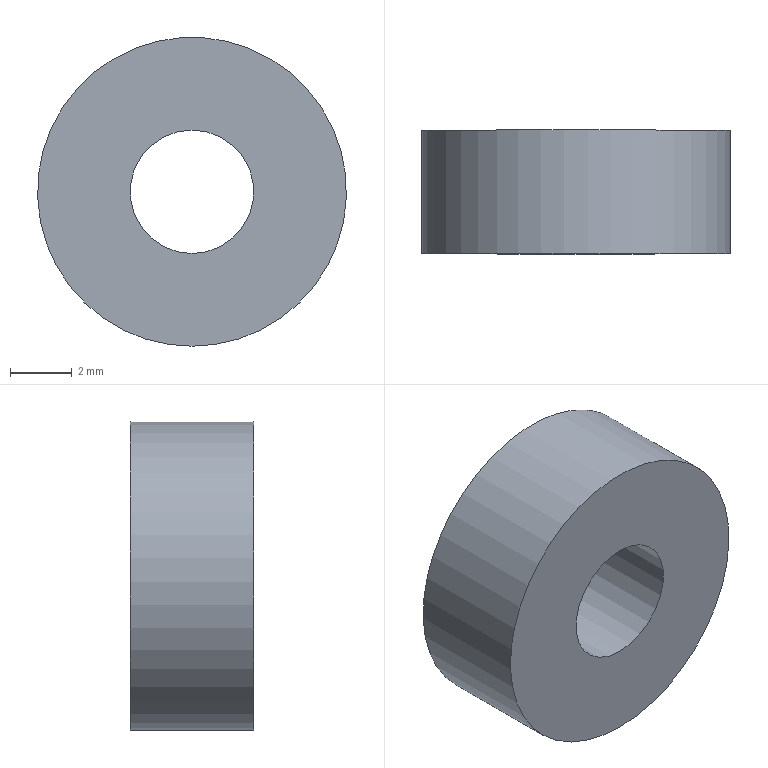Part | STEP file | Dodanie-wyci_gni_cie1 | 1 solid | 4 faces | box 10 x 4 x 10 mm | volume 263.894 mm3 | cylinder 2 | plane 2 | commonest cylinder face diameters 4 x1 10 x1
STEP:
#1=CARTESIAN_POINT('',(0.,0.,0.));
#2=DIRECTION('',(0.,0.,1.));
#3=DIRECTION('',(1.,0.,0.));
#4=AXIS2_PLACEMENT_3D('',#1,#2,#3);
#5=CARTESIAN_POINT('',(-99.682,73.388,-112.798));
#6=VERTEX_POINT('',#5);
#7=CARTESIAN_POINT('',(-99.682,69.388,-112.798));
#8=VERTEX_POINT('',#7);
#9=CARTESIAN_POINT('',(-99.682,73.388,-112.798));
#10=DIRECTION('',(0.,-1.,0.));
#11=VECTOR('',#10,1.);
#12=LINE('',#9,#11);
#13=CARTESIAN_POINT('',(-99.682,69.388,-107.798));
#14=DIRECTION('',(0.,1.,0.));
#15=DIRECTION('',(0.,0.,-1.));
#16=AXIS2_PLACEMENT_3D('',#13,#14,#15);
#17=CYLINDRICAL_SURFACE('',#16,5.);
#18=CARTESIAN_POINT('',(0.,4.));
#19=DIRECTION('',(0.,-1.));
#20=VECTOR('',#19,1.);
#21=LINE('',#18,#20);
#22=(GEOMETRIC_REPRESENTATION_CONTEXT(2)PARAMETRIC_REPRESENTATION_CONTEXT()REPRESENTATION_CONTEXT('',''));
#23=DEFINITIONAL_REPRESENTATION('',(#21),#22);
#24=PCURVE('',#17,#23);
#25=CARTESIAN_POINT('',(6.283,4.));
#26=DIRECTION('',(0.,-1.));
#27=VECTOR('',#26,1.);
#28=LINE('',#25,#27);
#29=(GEOMETRIC_REPRESENTATION_CONTEXT(2)PARAMETRIC_REPRESENTATION_CONTEXT()REPRESENTATION_CONTEXT('',''));
#30=DEFINITIONAL_REPRESENTATION('',(#28),#29);
#31=PCURVE('',#17,#30);
#32=SEAM_CURVE('',#12,(#24,#31),.PCURVE_S1.);
#33=EDGE_CURVE('',#6,#8,#32,.T.);
#34=ORIENTED_EDGE('',*,*,#33,.T.);
#35=CARTESIAN_POINT('',(-99.682,69.388,-107.798));
#36=DIRECTION('',(0.,1.,0.));
#37=DIRECTION('',(0.,0.,-1.));
#38=AXIS2_PLACEMENT_3D('',#35,#36,#37);
#39=CIRCLE('',#38,5.);
#40=CARTESIAN_POINT('',(0.,0.));
#41=DIRECTION('',(1.,0.));
#42=VECTOR('',#41,1.);
#43=LINE('',#40,#42);
#44=(GEOMETRIC_REPRESENTATION_CONTEXT(2)PARAMETRIC_REPRESENTATION_CONTEXT()REPRESENTATION_CONTEXT('',''));
#45=DEFINITIONAL_REPRESENTATION('',(#43),#44);
#46=PCURVE('',#17,#45);
#47=CARTESIAN_POINT('',(-99.682,69.388,-107.798));
#48=DIRECTION('',(0.,-1.,0.));
#49=DIRECTION('',(0.,0.,1.));
#50=AXIS2_PLACEMENT_3D('',#47,#48,#49);
#51=PLANE('',#50);
#52=CARTESIAN_POINT('',(-5.,0.));
#53=CARTESIAN_POINT('',(-5.,8.66));
#54=CARTESIAN_POINT('',(2.5,4.33));
#55=CARTESIAN_POINT('',(10.,0.));
#56=CARTESIAN_POINT('',(2.5,-4.33));
#57=CARTESIAN_POINT('',(-5.,-8.66));
#58=CARTESIAN_POINT('',(-5.,0.));
#59=(BOUNDED_CURVE()B_SPLINE_CURVE(2,(#52,#53,#54,#55,#56,#57,#58),.UNSPECIFIED.,.T.,.F.)B_SPLINE_CURVE_WITH_KNOTS((1,2,2,2,2,1),(-2.094,0.,2.094,4.189,6.283,8.378),.UNSPECIFIED.)CURVE()GEOMETRIC_REPRESENTATION_ITEM()RATIONAL_B_SPLINE_CURVE((1.,0.5,1.,0.5,1.,0.5,1.))REPRESENTATION_ITEM(''));
#60=(GEOMETRIC_REPRESENTATION_CONTEXT(2)PARAMETRIC_REPRESENTATION_CONTEXT()REPRESENTATION_CONTEXT('',''));
#61=DEFINITIONAL_REPRESENTATION('',(#59),#60);
#62=PCURVE('',#51,#61);
#63=SURFACE_CURVE('',#39,(#46,#62),.PCURVE_S1.);
#64=EDGE_CURVE('',#8,#8,#63,.T.);
#65=ORIENTED_EDGE('',*,*,#64,.T.);
#66=ORIENTED_EDGE('',*,*,#33,.F.);
#67=CARTESIAN_POINT('',(-99.682,73.388,-107.798));
#68=DIRECTION('',(0.,-1.,0.));
#69=DIRECTION('',(0.,0.,-1.));
#70=AXIS2_PLACEMENT_3D('',#67,#68,#69);
#71=CIRCLE('',#70,5.);
#72=CARTESIAN_POINT('',(6.283,4.));
#73=DIRECTION('',(-1.,0.));
#74=VECTOR('',#73,1.);
#75=LINE('',#72,#74);
#76=(GEOMETRIC_REPRESENTATION_CONTEXT(2)PARAMETRIC_REPRESENTATION_CONTEXT()REPRESENTATION_CONTEXT('',''));
#77=DEFINITIONAL_REPRESENTATION('',(#75),#76);
#78=PCURVE('',#17,#77);
#79=CARTESIAN_POINT('',(-99.682,73.388,-107.798));
#80=DIRECTION('',(0.,-1.,0.));
#81=DIRECTION('',(0.,0.,1.));
#82=AXIS2_PLACEMENT_3D('',#79,#80,#81);
#83=PLANE('',#82);
#84=CARTESIAN_POINT('',(0.,0.));
#85=DIRECTION('',(-1.,0.));
#86=AXIS2_PLACEMENT_2D('',#84,#85);
#87=CIRCLE('',#86,5.);
#88=(GEOMETRIC_REPRESENTATION_CONTEXT(2)PARAMETRIC_REPRESENTATION_CONTEXT()REPRESENTATION_CONTEXT('',''));
#89=DEFINITIONAL_REPRESENTATION('',(#87),#88);
#90=PCURVE('',#83,#89);
#91=SURFACE_CURVE('',#71,(#78,#90),.PCURVE_S1.);
#92=EDGE_CURVE('',#6,#6,#91,.T.);
#93=ORIENTED_EDGE('',*,*,#92,.T.);
#94=EDGE_LOOP('',(#34,#65,#66,#93));
#95=FACE_BOUND('',#94,.T.);
#96=ADVANCED_FACE('',(#95),#17,.T.);
#97=CARTESIAN_POINT('',(-99.682,69.388,-109.798));
#98=VERTEX_POINT('',#97);
#99=CARTESIAN_POINT('',(-99.682,69.388,-107.798));
#100=DIRECTION('',(0.,1.,0.));
#101=DIRECTION('',(0.,0.,-1.));
#102=AXIS2_PLACEMENT_3D('',#99,#100,#101);
#103=CIRCLE('',#102,2.);
#104=CARTESIAN_POINT('',(-99.682,69.388,-107.798));
#105=DIRECTION('',(0.,1.,0.));
#106=DIRECTION('',(0.,0.,-1.));
#107=AXIS2_PLACEMENT_3D('',#104,#105,#106);
#108=CYLINDRICAL_SURFACE('',#107,2.);
#109=CARTESIAN_POINT('',(0.,0.));
#110=DIRECTION('',(1.,0.));
#111=VECTOR('',#110,1.);
#112=LINE('',#109,#111);
#113=(GEOMETRIC_REPRESENTATION_CONTEXT(2)PARAMETRIC_REPRESENTATION_CONTEXT()REPRESENTATION_CONTEXT('',''));
#114=DEFINITIONAL_REPRESENTATION('',(#112),#113);
#115=PCURVE('',#108,#114);
#116=CARTESIAN_POINT('',(-2.,0.));
#117=CARTESIAN_POINT('',(-2.,3.464));
#118=CARTESIAN_POINT('',(1.,1.732));
#119=CARTESIAN_POINT('',(4.,0.));
#120=CARTESIAN_POINT('',(1.,-1.732));
#121=CARTESIAN_POINT('',(-2.,-3.464));
#122=CARTESIAN_POINT('',(-2.,0.));
#123=(BOUNDED_CURVE()B_SPLINE_CURVE(2,(#116,#117,#118,#119,#120,#121,#122),.UNSPECIFIED.,.T.,.F.)B_SPLINE_CURVE_WITH_KNOTS((1,2,2,2,2,1),(-2.094,0.,2.094,4.189,6.283,8.378),.UNSPECIFIED.)CURVE()GEOMETRIC_REPRESENTATION_ITEM()RATIONAL_B_SPLINE_CURVE((1.,0.5,1.,0.5,1.,0.5,1.))REPRESENTATION_ITEM(''));
#124=(GEOMETRIC_REPRESENTATION_CONTEXT(2)PARAMETRIC_REPRESENTATION_CONTEXT()REPRESENTATION_CONTEXT('',''));
#125=DEFINITIONAL_REPRESENTATION('',(#123),#124);
#126=PCURVE('',#51,#125);
#127=SURFACE_CURVE('',#103,(#115,#126),.PCURVE_S1.);
#128=EDGE_CURVE('',#98,#98,#127,.T.);
#129=ORIENTED_EDGE('',*,*,#128,.T.);
#130=CARTESIAN_POINT('',(-99.682,73.388,-109.798));
#131=VERTEX_POINT('',#130);
#132=CARTESIAN_POINT('',(-99.682,73.388,-109.798));
#133=DIRECTION('',(0.,-1.,0.));
#134=VECTOR('',#133,1.);
#135=LINE('',#132,#134);
#136=CARTESIAN_POINT('',(6.283,4.));
#137=DIRECTION('',(0.,-1.));
#138=VECTOR('',#137,1.);
#139=LINE('',#136,#138);
#140=(GEOMETRIC_REPRESENTATION_CONTEXT(2)PARAMETRIC_REPRESENTATION_CONTEXT()REPRESENTATION_CONTEXT('',''));
#141=DEFINITIONAL_REPRESENTATION('',(#139),#140);
#142=PCURVE('',#108,#141);
#143=CARTESIAN_POINT('',(0.,4.));
#144=DIRECTION('',(0.,-1.));
#145=VECTOR('',#144,1.);
#146=LINE('',#143,#145);
#147=(GEOMETRIC_REPRESENTATION_CONTEXT(2)PARAMETRIC_REPRESENTATION_CONTEXT()REPRESENTATION_CONTEXT('',''));
#148=DEFINITIONAL_REPRESENTATION('',(#146),#147);
#149=PCURVE('',#108,#148);
#150=SEAM_CURVE('',#135,(#142,#149),.PCURVE_S1.);
#151=EDGE_CURVE('',#131,#98,#150,.T.);
#152=ORIENTED_EDGE('',*,*,#151,.F.);
#153=CARTESIAN_POINT('',(-99.682,73.388,-107.798));
#154=DIRECTION('',(0.,1.,0.));
#155=DIRECTION('',(0.,0.,-1.));
#156=AXIS2_PLACEMENT_3D('',#153,#154,#155);
#157=CIRCLE('',#156,2.);
#158=CARTESIAN_POINT('',(0.,4.));
#159=DIRECTION('',(1.,0.));
#160=VECTOR('',#159,1.);
#161=LINE('',#158,#160);
#162=(GEOMETRIC_REPRESENTATION_CONTEXT(2)PARAMETRIC_REPRESENTATION_CONTEXT()REPRESENTATION_CONTEXT('',''));
#163=DEFINITIONAL_REPRESENTATION('',(#161),#162);
#164=PCURVE('',#108,#163);
#165=CARTESIAN_POINT('',(-2.,0.));
#166=CARTESIAN_POINT('',(-2.,3.464));
#167=CARTESIAN_POINT('',(1.,1.732));
#168=CARTESIAN_POINT('',(4.,0.));
#169=CARTESIAN_POINT('',(1.,-1.732));
#170=CARTESIAN_POINT('',(-2.,-3.464));
#171=CARTESIAN_POINT('',(-2.,0.));
#172=(BOUNDED_CURVE()B_SPLINE_CURVE(2,(#165,#166,#167,#168,#169,#170,#171),.UNSPECIFIED.,.T.,.F.)B_SPLINE_CURVE_WITH_KNOTS((1,2,2,2,2,1),(-2.094,0.,2.094,4.189,6.283,8.378),.UNSPECIFIED.)CURVE()GEOMETRIC_REPRESENTATION_ITEM()RATIONAL_B_SPLINE_CURVE((1.,0.5,1.,0.5,1.,0.5,1.))REPRESENTATION_ITEM(''));
#173=(GEOMETRIC_REPRESENTATION_CONTEXT(2)PARAMETRIC_REPRESENTATION_CONTEXT()REPRESENTATION_CONTEXT('',''));
#174=DEFINITIONAL_REPRESENTATION('',(#172),#173);
#175=PCURVE('',#83,#174);
#176=SURFACE_CURVE('',#157,(#164,#175),.PCURVE_S1.);
#177=EDGE_CURVE('',#131,#131,#176,.T.);
#178=ORIENTED_EDGE('',*,*,#177,.F.);
#179=ORIENTED_EDGE('',*,*,#151,.T.);
#180=EDGE_LOOP('',(#129,#152,#178,#179));
#181=FACE_BOUND('',#180,.F.);
#182=ADVANCED_FACE('',(#181),#108,.F.);
#183=ORIENTED_EDGE('',*,*,#177,.F.);
#184=EDGE_LOOP('',(#183));
#185=FACE_BOUND('',#184,.T.);
#186=ORIENTED_EDGE('',*,*,#92,.F.);
#187=EDGE_LOOP('',(#186));
#188=FACE_BOUND('',#187,.T.);
#189=ADVANCED_FACE('',(#185,#188),#83,.F.);
#190=ORIENTED_EDGE('',*,*,#128,.T.);
#191=EDGE_LOOP('',(#190));
#192=FACE_BOUND('',#191,.T.);
#193=ORIENTED_EDGE('',*,*,#64,.F.);
#194=EDGE_LOOP('',(#193));
#195=FACE_BOUND('',#194,.T.);
#196=ADVANCED_FACE('',(#192,#195),#51,.T.);
#197=CLOSED_SHELL('',(#96,#182,#189,#196));
#198=MANIFOLD_SOLID_BREP('',#197);
#199=(LENGTH_UNIT()NAMED_UNIT(*)SI_UNIT(.MILLI.,.METRE.));
#200=UNCERTAINTY_MEASURE_WITH_UNIT(LENGTH_MEASURE(0.0000001),#199,'','');
#201=(NAMED_UNIT(*)PLANE_ANGLE_UNIT()SI_UNIT($,.RADIAN.));
#202=(NAMED_UNIT(*)SI_UNIT($,.STERADIAN.)SOLID_ANGLE_UNIT());
#203=(GEOMETRIC_REPRESENTATION_CONTEXT(3)GLOBAL_UNCERTAINTY_ASSIGNED_CONTEXT((#200))GLOBAL_UNIT_ASSIGNED_CONTEXT((#199,#201,#202))REPRESENTATION_CONTEXT('',''));
#204=ADVANCED_BREP_SHAPE_REPRESENTATION('',(#4,#198),#203);